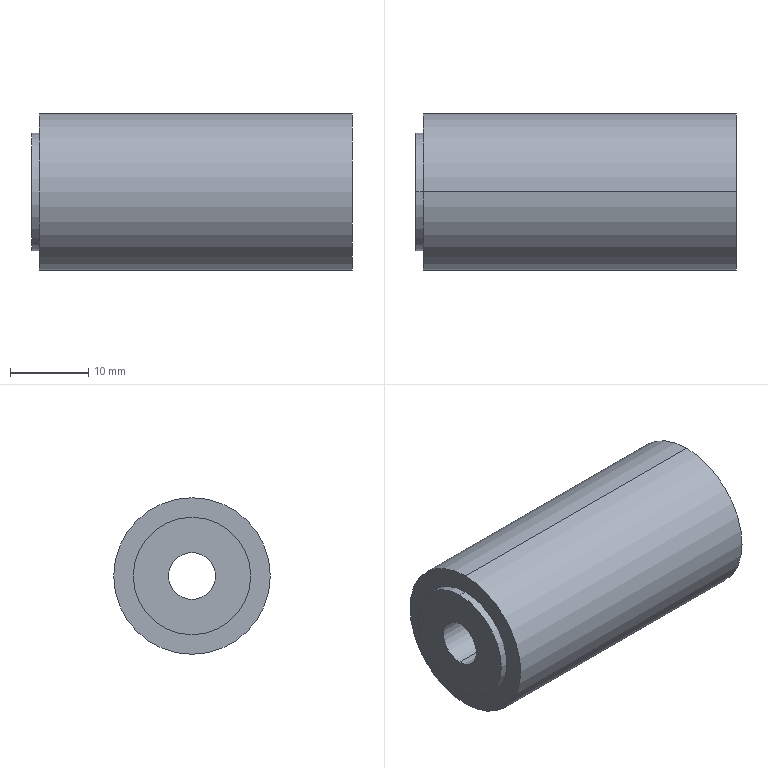Part | SolidWorks | features Extrusion 1, ICE 1 | 1 solid | 9 faces | box 41 x 20 x 20 mm | volume 11584 mm3 | cylinder 6 | plane 3 | commonest cylinder face diameters 6 x2 15 x2 20 x2
STEP:
#1=CARTESIAN_POINT('',(-1.,0.,7.5));
#2=VERTEX_POINT('',#1);
#3=CARTESIAN_POINT('',(-1.,0.,-7.5));
#4=VERTEX_POINT('',#3);
#5=CARTESIAN_POINT('',(-1.,0.,0.));
#6=DIRECTION('',(-1.,0.,0.));
#7=DIRECTION('',(0.,0.,1.));
#8=AXIS2_PLACEMENT_3D('',#5,#6,#7);
#9=CIRCLE('',#8,7.5);
#10=EDGE_CURVE('',#2,#4,#9,.T.);
#11=ORIENTED_EDGE('',*,*,#10,.F.);
#12=CARTESIAN_POINT('',(0.,0.,7.5));
#13=VERTEX_POINT('',#12);
#14=CARTESIAN_POINT('',(-1.,0.,7.5));
#15=DIRECTION('',(1.,0.,0.));
#16=VECTOR('',#15,1000.);
#17=LINE('',#14,#16);
#18=EDGE_CURVE('',#2,#13,#17,.T.);
#19=ORIENTED_EDGE('',*,*,#18,.T.);
#20=CARTESIAN_POINT('',(0.,0.,-7.5));
#21=VERTEX_POINT('',#20);
#22=CARTESIAN_POINT('',(0.,0.,0.));
#23=DIRECTION('',(-1.,0.,0.));
#24=DIRECTION('',(0.,0.,-1.));
#25=AXIS2_PLACEMENT_3D('',#22,#23,#24);
#26=CIRCLE('',#25,7.5);
#27=EDGE_CURVE('',#13,#21,#26,.T.);
#28=ORIENTED_EDGE('',*,*,#27,.T.);
#29=CARTESIAN_POINT('',(-1.,0.,-7.5));
#30=DIRECTION('',(1.,0.,0.));
#31=VECTOR('',#30,1000.);
#32=LINE('',#29,#31);
#33=EDGE_CURVE('',#4,#21,#32,.T.);
#34=ORIENTED_EDGE('',*,*,#33,.F.);
#35=EDGE_LOOP('',(#11,#19,#28,#34));
#36=FACE_OUTER_BOUND('',#35,.T.);
#37=CARTESIAN_POINT('',(-1.,0.,0.));
#38=DIRECTION('',(1.,0.,0.));
#39=DIRECTION('',(0.,0.,-1.));
#40=AXIS2_PLACEMENT_3D('',#37,#38,#39);
#41=CYLINDRICAL_SURFACE('',#40,7.5);
#42=ADVANCED_FACE('',(#36),#41,.T.);
#43=CARTESIAN_POINT('',(40.,0.,3.));
#44=VERTEX_POINT('',#43);
#45=CARTESIAN_POINT('',(40.,0.,-3.));
#46=VERTEX_POINT('',#45);
#47=CARTESIAN_POINT('',(40.,0.,0.));
#48=DIRECTION('',(1.,0.,0.));
#49=DIRECTION('',(0.,0.,-1.));
#50=AXIS2_PLACEMENT_3D('',#47,#48,#49);
#51=CIRCLE('',#50,3.);
#52=EDGE_CURVE('',#44,#46,#51,.T.);
#53=ORIENTED_EDGE('',*,*,#52,.T.);
#54=CARTESIAN_POINT('',(-1.,0.,-3.));
#55=VERTEX_POINT('',#54);
#56=CARTESIAN_POINT('',(40.,0.,-3.));
#57=DIRECTION('',(-1.,0.,0.));
#58=VECTOR('',#57,1000.);
#59=LINE('',#56,#58);
#60=EDGE_CURVE('',#46,#55,#59,.T.);
#61=ORIENTED_EDGE('',*,*,#60,.T.);
#62=CARTESIAN_POINT('',(-1.,0.,3.));
#63=VERTEX_POINT('',#62);
#64=CARTESIAN_POINT('',(-1.,0.,0.));
#65=DIRECTION('',(-1.,0.,0.));
#66=DIRECTION('',(0.,0.,1.));
#67=AXIS2_PLACEMENT_3D('',#64,#65,#66);
#68=CIRCLE('',#67,3.);
#69=EDGE_CURVE('',#55,#63,#68,.T.);
#70=ORIENTED_EDGE('',*,*,#69,.T.);
#71=CARTESIAN_POINT('',(40.,0.,3.));
#72=DIRECTION('',(-1.,0.,0.));
#73=VECTOR('',#72,1000.);
#74=LINE('',#71,#73);
#75=EDGE_CURVE('',#44,#63,#74,.T.);
#76=ORIENTED_EDGE('',*,*,#75,.F.);
#77=EDGE_LOOP('',(#53,#61,#70,#76));
#78=FACE_OUTER_BOUND('',#77,.T.);
#79=CARTESIAN_POINT('',(40.,0.,0.));
#80=DIRECTION('',(-1.,0.,0.));
#81=DIRECTION('',(0.,0.,1.));
#82=AXIS2_PLACEMENT_3D('',#79,#80,#81);
#83=CYLINDRICAL_SURFACE('',#82,3.);
#84=ADVANCED_FACE('',(#78),#83,.F.);
#85=CARTESIAN_POINT('',(40.,0.,-10.));
#86=VERTEX_POINT('',#85);
#87=CARTESIAN_POINT('',(40.,0.,10.));
#88=VERTEX_POINT('',#87);
#89=CARTESIAN_POINT('',(40.,0.,0.));
#90=DIRECTION('',(1.,0.,0.));
#91=DIRECTION('',(0.,0.,-1.));
#92=AXIS2_PLACEMENT_3D('',#89,#90,#91);
#93=CIRCLE('',#92,10.);
#94=EDGE_CURVE('',#86,#88,#93,.T.);
#95=ORIENTED_EDGE('',*,*,#94,.F.);
#96=CARTESIAN_POINT('',(0.,0.,-10.));
#97=VERTEX_POINT('',#96);
#98=CARTESIAN_POINT('',(40.,0.,-10.));
#99=DIRECTION('',(-1.,0.,0.));
#100=VECTOR('',#99,1000.);
#101=LINE('',#98,#100);
#102=EDGE_CURVE('',#86,#97,#101,.T.);
#103=ORIENTED_EDGE('',*,*,#102,.T.);
#104=CARTESIAN_POINT('',(0.,0.,10.));
#105=VERTEX_POINT('',#104);
#106=CARTESIAN_POINT('',(0.,0.,0.));
#107=DIRECTION('',(1.,0.,0.));
#108=DIRECTION('',(0.,0.,-1.));
#109=AXIS2_PLACEMENT_3D('',#106,#107,#108);
#110=CIRCLE('',#109,10.);
#111=EDGE_CURVE('',#97,#105,#110,.T.);
#112=ORIENTED_EDGE('',*,*,#111,.T.);
#113=CARTESIAN_POINT('',(40.,0.,10.));
#114=DIRECTION('',(-1.,0.,0.));
#115=VECTOR('',#114,1000.);
#116=LINE('',#113,#115);
#117=EDGE_CURVE('',#88,#105,#116,.T.);
#118=ORIENTED_EDGE('',*,*,#117,.F.);
#119=EDGE_LOOP('',(#95,#103,#112,#118));
#120=FACE_OUTER_BOUND('',#119,.T.);
#121=CARTESIAN_POINT('',(40.,0.,0.));
#122=DIRECTION('',(-1.,0.,0.));
#123=DIRECTION('',(0.,0.,1.));
#124=AXIS2_PLACEMENT_3D('',#121,#122,#123);
#125=CYLINDRICAL_SURFACE('',#124,10.);
#126=ADVANCED_FACE('',(#120),#125,.T.);
#127=CARTESIAN_POINT('',(0.,0.,0.));
#128=DIRECTION('',(1.,0.,0.));
#129=DIRECTION('',(0.,0.,-1.));
#130=AXIS2_PLACEMENT_3D('',#127,#128,#129);
#131=CIRCLE('',#130,10.);
#132=EDGE_CURVE('',#105,#97,#131,.T.);
#133=ORIENTED_EDGE('',*,*,#132,.F.);
#134=ORIENTED_EDGE('',*,*,#111,.F.);
#135=EDGE_LOOP('',(#133,#134));
#136=FACE_OUTER_BOUND('',#135,.T.);
#137=CARTESIAN_POINT('',(0.,0.,0.));
#138=DIRECTION('',(-1.,0.,0.));
#139=DIRECTION('',(0.,0.,-1.));
#140=AXIS2_PLACEMENT_3D('',#137,#138,#139);
#141=CIRCLE('',#140,7.5);
#142=EDGE_CURVE('',#21,#13,#141,.T.);
#143=ORIENTED_EDGE('',*,*,#142,.F.);
#144=ORIENTED_EDGE('',*,*,#27,.F.);
#145=EDGE_LOOP('',(#143,#144));
#146=FACE_BOUND('',#145,.T.);
#147=CARTESIAN_POINT('',(0.,0.,0.));
#148=DIRECTION('',(1.,0.,0.));
#149=DIRECTION('',(0.,0.,-1.));
#150=AXIS2_PLACEMENT_3D('',#147,#148,#149);
#151=PLANE('',#150);
#152=ADVANCED_FACE('',(#136,#146),#151,.F.);
#153=CARTESIAN_POINT('',(40.,0.,0.));
#154=DIRECTION('',(1.,0.,0.));
#155=DIRECTION('',(0.,0.,-1.));
#156=AXIS2_PLACEMENT_3D('',#153,#154,#155);
#157=CIRCLE('',#156,10.);
#158=EDGE_CURVE('',#88,#86,#157,.T.);
#159=ORIENTED_EDGE('',*,*,#158,.T.);
#160=ORIENTED_EDGE('',*,*,#94,.T.);
#161=EDGE_LOOP('',(#159,#160));
#162=FACE_OUTER_BOUND('',#161,.T.);
#163=ORIENTED_EDGE('',*,*,#52,.F.);
#164=CARTESIAN_POINT('',(40.,0.,0.));
#165=DIRECTION('',(1.,0.,0.));
#166=DIRECTION('',(0.,0.,-1.));
#167=AXIS2_PLACEMENT_3D('',#164,#165,#166);
#168=CIRCLE('',#167,3.);
#169=EDGE_CURVE('',#46,#44,#168,.T.);
#170=ORIENTED_EDGE('',*,*,#169,.F.);
#171=EDGE_LOOP('',(#163,#170));
#172=FACE_BOUND('',#171,.T.);
#173=CARTESIAN_POINT('',(40.,0.,0.));
#174=DIRECTION('',(1.,0.,0.));
#175=DIRECTION('',(0.,0.,-1.));
#176=AXIS2_PLACEMENT_3D('',#173,#174,#175);
#177=PLANE('',#176);
#178=ADVANCED_FACE('',(#162,#172),#177,.T.);
#179=ORIENTED_EDGE('',*,*,#102,.F.);
#180=ORIENTED_EDGE('',*,*,#158,.F.);
#181=ORIENTED_EDGE('',*,*,#117,.T.);
#182=ORIENTED_EDGE('',*,*,#132,.T.);
#183=EDGE_LOOP('',(#179,#180,#181,#182));
#184=FACE_OUTER_BOUND('',#183,.T.);
#185=CARTESIAN_POINT('',(40.,0.,0.));
#186=DIRECTION('',(-1.,0.,0.));
#187=DIRECTION('',(0.,0.,1.));
#188=AXIS2_PLACEMENT_3D('',#185,#186,#187);
#189=CYLINDRICAL_SURFACE('',#188,10.);
#190=ADVANCED_FACE('',(#184),#189,.T.);
#191=ORIENTED_EDGE('',*,*,#60,.F.);
#192=ORIENTED_EDGE('',*,*,#169,.T.);
#193=ORIENTED_EDGE('',*,*,#75,.T.);
#194=CARTESIAN_POINT('',(-1.,0.,0.));
#195=DIRECTION('',(-1.,0.,0.));
#196=DIRECTION('',(0.,0.,1.));
#197=AXIS2_PLACEMENT_3D('',#194,#195,#196);
#198=CIRCLE('',#197,3.);
#199=EDGE_CURVE('',#63,#55,#198,.T.);
#200=ORIENTED_EDGE('',*,*,#199,.T.);
#201=EDGE_LOOP('',(#191,#192,#193,#200));
#202=FACE_OUTER_BOUND('',#201,.T.);
#203=CARTESIAN_POINT('',(40.,0.,0.));
#204=DIRECTION('',(-1.,0.,0.));
#205=DIRECTION('',(0.,0.,1.));
#206=AXIS2_PLACEMENT_3D('',#203,#204,#205);
#207=CYLINDRICAL_SURFACE('',#206,3.);
#208=ADVANCED_FACE('',(#202),#207,.F.);
#209=CARTESIAN_POINT('',(-1.,0.,0.));
#210=DIRECTION('',(-1.,0.,0.));
#211=DIRECTION('',(0.,0.,1.));
#212=AXIS2_PLACEMENT_3D('',#209,#210,#211);
#213=CIRCLE('',#212,7.5);
#214=EDGE_CURVE('',#4,#2,#213,.T.);
#215=ORIENTED_EDGE('',*,*,#214,.T.);
#216=ORIENTED_EDGE('',*,*,#10,.T.);
#217=EDGE_LOOP('',(#215,#216));
#218=FACE_OUTER_BOUND('',#217,.T.);
#219=ORIENTED_EDGE('',*,*,#199,.F.);
#220=ORIENTED_EDGE('',*,*,#69,.F.);
#221=EDGE_LOOP('',(#219,#220));
#222=FACE_BOUND('',#221,.T.);
#223=CARTESIAN_POINT('',(-1.,0.,0.));
#224=DIRECTION('',(-1.,0.,0.));
#225=DIRECTION('',(0.,0.,1.));
#226=AXIS2_PLACEMENT_3D('',#223,#224,#225);
#227=PLANE('',#226);
#228=ADVANCED_FACE('',(#218,#222),#227,.T.);
#229=ORIENTED_EDGE('',*,*,#18,.F.);
#230=ORIENTED_EDGE('',*,*,#214,.F.);
#231=ORIENTED_EDGE('',*,*,#33,.T.);
#232=ORIENTED_EDGE('',*,*,#142,.T.);
#233=EDGE_LOOP('',(#229,#230,#231,#232));
#234=FACE_OUTER_BOUND('',#233,.T.);
#235=CARTESIAN_POINT('',(-1.,0.,0.));
#236=DIRECTION('',(1.,0.,0.));
#237=DIRECTION('',(0.,0.,-1.));
#238=AXIS2_PLACEMENT_3D('',#235,#236,#237);
#239=CYLINDRICAL_SURFACE('',#238,7.5);
#240=ADVANCED_FACE('',(#234),#239,.T.);
#241=CLOSED_SHELL('',(#42,#84,#126,#152,#178,#190,#208,#228,#240));
#242=MANIFOLD_SOLID_BREP('',#241);
#243=CARTESIAN_POINT('',(0.,0.,0.));
#244=DIRECTION('',(0.,0.,1.));
#245=DIRECTION('',(1.,0.,0.));
#246=AXIS2_PLACEMENT_3D('',#243,#244,#245);
#247=(LENGTH_UNIT()NAMED_UNIT(*)SI_UNIT(.MILLI.,.METRE.));
#248=UNCERTAINTY_MEASURE_WITH_UNIT(LENGTH_MEASURE(0.00001),#247,'','');
#249=(NAMED_UNIT(*)PLANE_ANGLE_UNIT()SI_UNIT($,.RADIAN.));
#250=(NAMED_UNIT(*)SI_UNIT($,.STERADIAN.)SOLID_ANGLE_UNIT());
#251=(GEOMETRIC_REPRESENTATION_CONTEXT(3)GLOBAL_UNCERTAINTY_ASSIGNED_CONTEXT((#248))GLOBAL_UNIT_ASSIGNED_CONTEXT((#247,#249,#250))REPRESENTATION_CONTEXT('',''));
#252=ADVANCED_BREP_SHAPE_REPRESENTATION('',(#242,#246),#251);